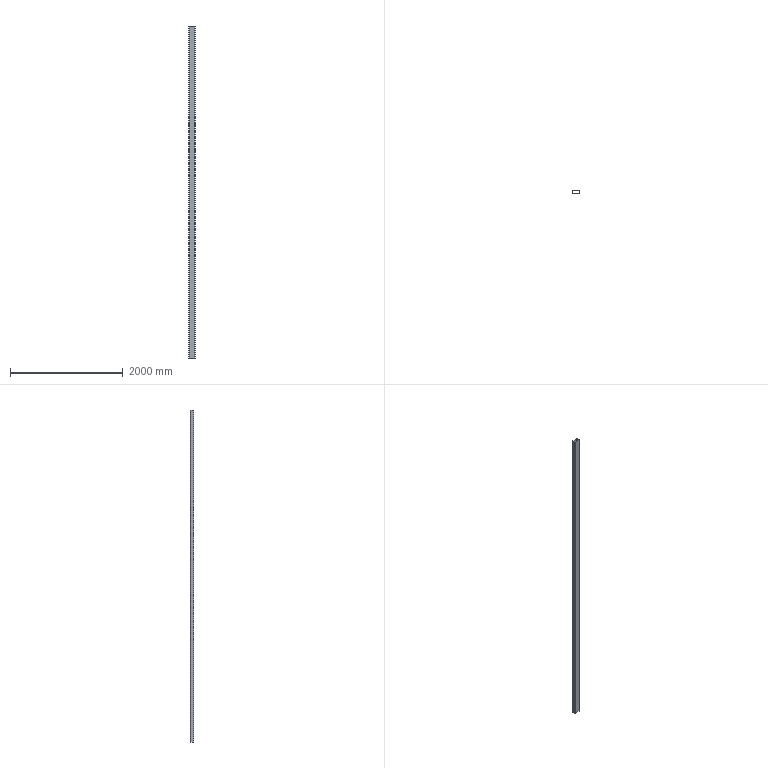Part | SolidWorks | features Extrusion 1 | 1 solid | 18 faces | box 120 x 60 x 5880 mm | volume 9617442 mm3 | plane 10 | cylinder 8 | commonest cylinder face diameters 10 x4 20 x4
STEP:
#1=CARTESIAN_POINT('',(110.,0.,5880.));
#2=VERTEX_POINT('',#1);
#3=CARTESIAN_POINT('',(120.,10.,5880.));
#4=VERTEX_POINT('',#3);
#5=CARTESIAN_POINT('',(110.,10.,5880.));
#6=DIRECTION('',(0.,0.,1.));
#7=DIRECTION('',(-1.,0.,0.));
#8=AXIS2_PLACEMENT_3D('',#5,#6,#7);
#9=CIRCLE('',#8,10.);
#10=EDGE_CURVE('',#2,#4,#9,.T.);
#11=ORIENTED_EDGE('',*,*,#10,.T.);
#12=CARTESIAN_POINT('',(120.,50.,5880.));
#13=VERTEX_POINT('',#12);
#14=CARTESIAN_POINT('',(120.,10.,5880.));
#15=DIRECTION('',(0.,1.,0.));
#16=VECTOR('',#15,1000.);
#17=LINE('',#14,#16);
#18=EDGE_CURVE('',#4,#13,#17,.T.);
#19=ORIENTED_EDGE('',*,*,#18,.T.);
#20=CARTESIAN_POINT('',(110.,60.,5880.));
#21=VERTEX_POINT('',#20);
#22=CARTESIAN_POINT('',(110.,50.,5880.));
#23=DIRECTION('',(0.,0.,1.));
#24=DIRECTION('',(1.,0.,0.));
#25=AXIS2_PLACEMENT_3D('',#22,#23,#24);
#26=CIRCLE('',#25,10.);
#27=EDGE_CURVE('',#13,#21,#26,.T.);
#28=ORIENTED_EDGE('',*,*,#27,.T.);
#29=CARTESIAN_POINT('',(10.,60.,5880.));
#30=VERTEX_POINT('',#29);
#31=CARTESIAN_POINT('',(10.,60.,5880.));
#32=DIRECTION('',(-1.,0.,0.));
#33=VECTOR('',#32,1000.);
#34=LINE('',#31,#33);
#35=EDGE_CURVE('',#21,#30,#34,.T.);
#36=ORIENTED_EDGE('',*,*,#35,.T.);
#37=CARTESIAN_POINT('',(0.,50.,5880.));
#38=VERTEX_POINT('',#37);
#39=CARTESIAN_POINT('',(10.,50.,5880.));
#40=DIRECTION('',(0.,0.,1.));
#41=DIRECTION('',(-1.,0.,0.));
#42=AXIS2_PLACEMENT_3D('',#39,#40,#41);
#43=CIRCLE('',#42,10.);
#44=EDGE_CURVE('',#30,#38,#43,.T.);
#45=ORIENTED_EDGE('',*,*,#44,.T.);
#46=CARTESIAN_POINT('',(0.,10.,5880.));
#47=VERTEX_POINT('',#46);
#48=CARTESIAN_POINT('',(0.,10.,5880.));
#49=DIRECTION('',(0.,-1.,0.));
#50=VECTOR('',#49,1000.);
#51=LINE('',#48,#50);
#52=EDGE_CURVE('',#38,#47,#51,.T.);
#53=ORIENTED_EDGE('',*,*,#52,.T.);
#54=CARTESIAN_POINT('',(10.,0.,5880.));
#55=VERTEX_POINT('',#54);
#56=CARTESIAN_POINT('',(10.,10.,5880.));
#57=DIRECTION('',(0.,0.,1.));
#58=DIRECTION('',(-1.,0.,0.));
#59=AXIS2_PLACEMENT_3D('',#56,#57,#58);
#60=CIRCLE('',#59,10.);
#61=EDGE_CURVE('',#47,#55,#60,.T.);
#62=ORIENTED_EDGE('',*,*,#61,.T.);
#63=CARTESIAN_POINT('',(10.,0.,5880.));
#64=DIRECTION('',(1.,0.,0.));
#65=VECTOR('',#64,1000.);
#66=LINE('',#63,#65);
#67=EDGE_CURVE('',#55,#2,#66,.T.);
#68=ORIENTED_EDGE('',*,*,#67,.T.);
#69=EDGE_LOOP('',(#11,#19,#28,#36,#45,#53,#62,#68));
#70=FACE_OUTER_BOUND('',#69,.T.);
#71=CARTESIAN_POINT('',(10.,55.,5880.));
#72=VERTEX_POINT('',#71);
#73=CARTESIAN_POINT('',(5.,50.,5880.));
#74=VERTEX_POINT('',#73);
#75=CARTESIAN_POINT('',(10.,50.,5880.));
#76=DIRECTION('',(0.,0.,1.));
#77=DIRECTION('',(-1.,0.,0.));
#78=AXIS2_PLACEMENT_3D('',#75,#76,#77);
#79=CIRCLE('',#78,5.);
#80=EDGE_CURVE('',#72,#74,#79,.T.);
#81=ORIENTED_EDGE('',*,*,#80,.F.);
#82=CARTESIAN_POINT('',(110.,55.,5880.));
#83=VERTEX_POINT('',#82);
#84=CARTESIAN_POINT('',(10.,55.,5880.));
#85=DIRECTION('',(-1.,0.,0.));
#86=VECTOR('',#85,1000.);
#87=LINE('',#84,#86);
#88=EDGE_CURVE('',#83,#72,#87,.T.);
#89=ORIENTED_EDGE('',*,*,#88,.F.);
#90=CARTESIAN_POINT('',(115.,50.,5880.));
#91=VERTEX_POINT('',#90);
#92=CARTESIAN_POINT('',(110.,50.,5880.));
#93=DIRECTION('',(0.,0.,1.));
#94=DIRECTION('',(1.,0.,0.));
#95=AXIS2_PLACEMENT_3D('',#92,#93,#94);
#96=CIRCLE('',#95,5.);
#97=EDGE_CURVE('',#91,#83,#96,.T.);
#98=ORIENTED_EDGE('',*,*,#97,.F.);
#99=CARTESIAN_POINT('',(115.,10.,5880.));
#100=VERTEX_POINT('',#99);
#101=CARTESIAN_POINT('',(115.,10.,5880.));
#102=DIRECTION('',(0.,1.,0.));
#103=VECTOR('',#102,1000.);
#104=LINE('',#101,#103);
#105=EDGE_CURVE('',#100,#91,#104,.T.);
#106=ORIENTED_EDGE('',*,*,#105,.F.);
#107=CARTESIAN_POINT('',(110.,5.,5880.));
#108=VERTEX_POINT('',#107);
#109=CARTESIAN_POINT('',(110.,10.,5880.));
#110=DIRECTION('',(0.,0.,1.));
#111=DIRECTION('',(-1.,0.,0.));
#112=AXIS2_PLACEMENT_3D('',#109,#110,#111);
#113=CIRCLE('',#112,5.);
#114=EDGE_CURVE('',#108,#100,#113,.T.);
#115=ORIENTED_EDGE('',*,*,#114,.F.);
#116=CARTESIAN_POINT('',(10.,5.,5880.));
#117=VERTEX_POINT('',#116);
#118=CARTESIAN_POINT('',(10.,5.,5880.));
#119=DIRECTION('',(1.,0.,0.));
#120=VECTOR('',#119,1000.);
#121=LINE('',#118,#120);
#122=EDGE_CURVE('',#117,#108,#121,.T.);
#123=ORIENTED_EDGE('',*,*,#122,.F.);
#124=CARTESIAN_POINT('',(5.,10.,5880.));
#125=VERTEX_POINT('',#124);
#126=CARTESIAN_POINT('',(10.,10.,5880.));
#127=DIRECTION('',(0.,0.,1.));
#128=DIRECTION('',(-1.,0.,0.));
#129=AXIS2_PLACEMENT_3D('',#126,#127,#128);
#130=CIRCLE('',#129,5.);
#131=EDGE_CURVE('',#125,#117,#130,.T.);
#132=ORIENTED_EDGE('',*,*,#131,.F.);
#133=CARTESIAN_POINT('',(5.,10.,5880.));
#134=DIRECTION('',(0.,-1.,0.));
#135=VECTOR('',#134,1000.);
#136=LINE('',#133,#135);
#137=EDGE_CURVE('',#74,#125,#136,.T.);
#138=ORIENTED_EDGE('',*,*,#137,.F.);
#139=EDGE_LOOP('',(#81,#89,#98,#106,#115,#123,#132,#138));
#140=FACE_BOUND('',#139,.T.);
#141=CARTESIAN_POINT('',(110.,10.,5880.));
#142=DIRECTION('',(0.,0.,-1.));
#143=DIRECTION('',(-1.,0.,0.));
#144=AXIS2_PLACEMENT_3D('',#141,#142,#143);
#145=PLANE('',#144);
#146=ADVANCED_FACE('',(#70,#140),#145,.F.);
#147=CARTESIAN_POINT('',(110.,0.,0.));
#148=VERTEX_POINT('',#147);
#149=CARTESIAN_POINT('',(120.,10.,0.));
#150=VERTEX_POINT('',#149);
#151=CARTESIAN_POINT('',(110.,10.,0.));
#152=DIRECTION('',(0.,0.,1.));
#153=DIRECTION('',(-1.,0.,0.));
#154=AXIS2_PLACEMENT_3D('',#151,#152,#153);
#155=CIRCLE('',#154,10.);
#156=EDGE_CURVE('',#148,#150,#155,.T.);
#157=ORIENTED_EDGE('',*,*,#156,.F.);
#158=CARTESIAN_POINT('',(10.,0.,0.));
#159=VERTEX_POINT('',#158);
#160=CARTESIAN_POINT('',(10.,0.,0.));
#161=DIRECTION('',(1.,0.,0.));
#162=VECTOR('',#161,1000.);
#163=LINE('',#160,#162);
#164=EDGE_CURVE('',#159,#148,#163,.T.);
#165=ORIENTED_EDGE('',*,*,#164,.F.);
#166=CARTESIAN_POINT('',(0.,10.,0.));
#167=VERTEX_POINT('',#166);
#168=CARTESIAN_POINT('',(10.,10.,0.));
#169=DIRECTION('',(0.,0.,1.));
#170=DIRECTION('',(-1.,0.,0.));
#171=AXIS2_PLACEMENT_3D('',#168,#169,#170);
#172=CIRCLE('',#171,10.);
#173=EDGE_CURVE('',#167,#159,#172,.T.);
#174=ORIENTED_EDGE('',*,*,#173,.F.);
#175=CARTESIAN_POINT('',(0.,50.,0.));
#176=VERTEX_POINT('',#175);
#177=CARTESIAN_POINT('',(0.,10.,0.));
#178=DIRECTION('',(0.,-1.,0.));
#179=VECTOR('',#178,1000.);
#180=LINE('',#177,#179);
#181=EDGE_CURVE('',#176,#167,#180,.T.);
#182=ORIENTED_EDGE('',*,*,#181,.F.);
#183=CARTESIAN_POINT('',(10.,60.,0.));
#184=VERTEX_POINT('',#183);
#185=CARTESIAN_POINT('',(10.,50.,0.));
#186=DIRECTION('',(0.,0.,1.));
#187=DIRECTION('',(-1.,0.,0.));
#188=AXIS2_PLACEMENT_3D('',#185,#186,#187);
#189=CIRCLE('',#188,10.);
#190=EDGE_CURVE('',#184,#176,#189,.T.);
#191=ORIENTED_EDGE('',*,*,#190,.F.);
#192=CARTESIAN_POINT('',(110.,60.,0.));
#193=VERTEX_POINT('',#192);
#194=CARTESIAN_POINT('',(10.,60.,0.));
#195=DIRECTION('',(-1.,0.,0.));
#196=VECTOR('',#195,1000.);
#197=LINE('',#194,#196);
#198=EDGE_CURVE('',#193,#184,#197,.T.);
#199=ORIENTED_EDGE('',*,*,#198,.F.);
#200=CARTESIAN_POINT('',(120.,50.,0.));
#201=VERTEX_POINT('',#200);
#202=CARTESIAN_POINT('',(110.,50.,0.));
#203=DIRECTION('',(0.,0.,1.));
#204=DIRECTION('',(1.,0.,0.));
#205=AXIS2_PLACEMENT_3D('',#202,#203,#204);
#206=CIRCLE('',#205,10.);
#207=EDGE_CURVE('',#201,#193,#206,.T.);
#208=ORIENTED_EDGE('',*,*,#207,.F.);
#209=CARTESIAN_POINT('',(120.,10.,0.));
#210=DIRECTION('',(0.,1.,0.));
#211=VECTOR('',#210,1000.);
#212=LINE('',#209,#211);
#213=EDGE_CURVE('',#150,#201,#212,.T.);
#214=ORIENTED_EDGE('',*,*,#213,.F.);
#215=EDGE_LOOP('',(#157,#165,#174,#182,#191,#199,#208,#214));
#216=FACE_OUTER_BOUND('',#215,.T.);
#217=CARTESIAN_POINT('',(110.,55.,0.));
#218=VERTEX_POINT('',#217);
#219=CARTESIAN_POINT('',(10.,55.,0.));
#220=VERTEX_POINT('',#219);
#221=CARTESIAN_POINT('',(10.,55.,0.));
#222=DIRECTION('',(-1.,0.,0.));
#223=VECTOR('',#222,1000.);
#224=LINE('',#221,#223);
#225=EDGE_CURVE('',#218,#220,#224,.T.);
#226=ORIENTED_EDGE('',*,*,#225,.T.);
#227=CARTESIAN_POINT('',(5.,50.,0.));
#228=VERTEX_POINT('',#227);
#229=CARTESIAN_POINT('',(10.,50.,0.));
#230=DIRECTION('',(0.,0.,1.));
#231=DIRECTION('',(-1.,0.,0.));
#232=AXIS2_PLACEMENT_3D('',#229,#230,#231);
#233=CIRCLE('',#232,5.);
#234=EDGE_CURVE('',#220,#228,#233,.T.);
#235=ORIENTED_EDGE('',*,*,#234,.T.);
#236=CARTESIAN_POINT('',(5.,10.,0.));
#237=VERTEX_POINT('',#236);
#238=CARTESIAN_POINT('',(5.,10.,0.));
#239=DIRECTION('',(0.,-1.,0.));
#240=VECTOR('',#239,1000.);
#241=LINE('',#238,#240);
#242=EDGE_CURVE('',#228,#237,#241,.T.);
#243=ORIENTED_EDGE('',*,*,#242,.T.);
#244=CARTESIAN_POINT('',(10.,5.,0.));
#245=VERTEX_POINT('',#244);
#246=CARTESIAN_POINT('',(10.,10.,0.));
#247=DIRECTION('',(0.,0.,1.));
#248=DIRECTION('',(-1.,0.,0.));
#249=AXIS2_PLACEMENT_3D('',#246,#247,#248);
#250=CIRCLE('',#249,5.);
#251=EDGE_CURVE('',#237,#245,#250,.T.);
#252=ORIENTED_EDGE('',*,*,#251,.T.);
#253=CARTESIAN_POINT('',(110.,5.,0.));
#254=VERTEX_POINT('',#253);
#255=CARTESIAN_POINT('',(10.,5.,0.));
#256=DIRECTION('',(1.,0.,0.));
#257=VECTOR('',#256,1000.);
#258=LINE('',#255,#257);
#259=EDGE_CURVE('',#245,#254,#258,.T.);
#260=ORIENTED_EDGE('',*,*,#259,.T.);
#261=CARTESIAN_POINT('',(115.,10.,0.));
#262=VERTEX_POINT('',#261);
#263=CARTESIAN_POINT('',(110.,10.,0.));
#264=DIRECTION('',(0.,0.,1.));
#265=DIRECTION('',(-1.,0.,0.));
#266=AXIS2_PLACEMENT_3D('',#263,#264,#265);
#267=CIRCLE('',#266,5.);
#268=EDGE_CURVE('',#254,#262,#267,.T.);
#269=ORIENTED_EDGE('',*,*,#268,.T.);
#270=CARTESIAN_POINT('',(115.,50.,0.));
#271=VERTEX_POINT('',#270);
#272=CARTESIAN_POINT('',(115.,10.,0.));
#273=DIRECTION('',(0.,1.,0.));
#274=VECTOR('',#273,1000.);
#275=LINE('',#272,#274);
#276=EDGE_CURVE('',#262,#271,#275,.T.);
#277=ORIENTED_EDGE('',*,*,#276,.T.);
#278=CARTESIAN_POINT('',(110.,50.,0.));
#279=DIRECTION('',(0.,0.,1.));
#280=DIRECTION('',(1.,0.,0.));
#281=AXIS2_PLACEMENT_3D('',#278,#279,#280);
#282=CIRCLE('',#281,5.);
#283=EDGE_CURVE('',#271,#218,#282,.T.);
#284=ORIENTED_EDGE('',*,*,#283,.T.);
#285=EDGE_LOOP('',(#226,#235,#243,#252,#260,#269,#277,#284));
#286=FACE_BOUND('',#285,.T.);
#287=CARTESIAN_POINT('',(110.,10.,0.));
#288=DIRECTION('',(0.,0.,-1.));
#289=DIRECTION('',(-1.,0.,0.));
#290=AXIS2_PLACEMENT_3D('',#287,#288,#289);
#291=PLANE('',#290);
#292=ADVANCED_FACE('',(#216,#286),#291,.T.);
#293=ORIENTED_EDGE('',*,*,#156,.T.);
#294=CARTESIAN_POINT('',(120.,10.,5880.));
#295=DIRECTION('',(0.,0.,-1.));
#296=VECTOR('',#295,1000.);
#297=LINE('',#294,#296);
#298=EDGE_CURVE('',#4,#150,#297,.T.);
#299=ORIENTED_EDGE('',*,*,#298,.F.);
#300=ORIENTED_EDGE('',*,*,#10,.F.);
#301=CARTESIAN_POINT('',(110.,0.,5880.));
#302=DIRECTION('',(0.,0.,-1.));
#303=VECTOR('',#302,1000.);
#304=LINE('',#301,#303);
#305=EDGE_CURVE('',#2,#148,#304,.T.);
#306=ORIENTED_EDGE('',*,*,#305,.T.);
#307=EDGE_LOOP('',(#293,#299,#300,#306));
#308=FACE_OUTER_BOUND('',#307,.T.);
#309=CARTESIAN_POINT('',(110.,10.,5880.));
#310=DIRECTION('',(0.,0.,-1.));
#311=DIRECTION('',(-1.,0.,0.));
#312=AXIS2_PLACEMENT_3D('',#309,#310,#311);
#313=CYLINDRICAL_SURFACE('',#312,10.);
#314=ADVANCED_FACE('',(#308),#313,.T.);
#315=ORIENTED_EDGE('',*,*,#213,.T.);
#316=CARTESIAN_POINT('',(120.,50.,5880.));
#317=DIRECTION('',(0.,0.,-1.));
#318=VECTOR('',#317,1000.);
#319=LINE('',#316,#318);
#320=EDGE_CURVE('',#13,#201,#319,.T.);
#321=ORIENTED_EDGE('',*,*,#320,.F.);
#322=ORIENTED_EDGE('',*,*,#18,.F.);
#323=ORIENTED_EDGE('',*,*,#298,.T.);
#324=EDGE_LOOP('',(#315,#321,#322,#323));
#325=FACE_OUTER_BOUND('',#324,.T.);
#326=CARTESIAN_POINT('',(120.,10.,5880.));
#327=DIRECTION('',(-1.,0.,0.));
#328=DIRECTION('',(0.,-1.,0.));
#329=AXIS2_PLACEMENT_3D('',#326,#327,#328);
#330=PLANE('',#329);
#331=ADVANCED_FACE('',(#325),#330,.F.);
#332=ORIENTED_EDGE('',*,*,#207,.T.);
#333=CARTESIAN_POINT('',(110.,60.,5880.));
#334=DIRECTION('',(0.,0.,-1.));
#335=VECTOR('',#334,1000.);
#336=LINE('',#333,#335);
#337=EDGE_CURVE('',#21,#193,#336,.T.);
#338=ORIENTED_EDGE('',*,*,#337,.F.);
#339=ORIENTED_EDGE('',*,*,#27,.F.);
#340=ORIENTED_EDGE('',*,*,#320,.T.);
#341=EDGE_LOOP('',(#332,#338,#339,#340));
#342=FACE_OUTER_BOUND('',#341,.T.);
#343=CARTESIAN_POINT('',(110.,50.,5880.));
#344=DIRECTION('',(0.,0.,-1.));
#345=DIRECTION('',(-1.,0.,0.));
#346=AXIS2_PLACEMENT_3D('',#343,#344,#345);
#347=CYLINDRICAL_SURFACE('',#346,10.);
#348=ADVANCED_FACE('',(#342),#347,.T.);
#349=ORIENTED_EDGE('',*,*,#198,.T.);
#350=CARTESIAN_POINT('',(10.,60.,5880.));
#351=DIRECTION('',(0.,0.,-1.));
#352=VECTOR('',#351,1000.);
#353=LINE('',#350,#352);
#354=EDGE_CURVE('',#30,#184,#353,.T.);
#355=ORIENTED_EDGE('',*,*,#354,.F.);
#356=ORIENTED_EDGE('',*,*,#35,.F.);
#357=ORIENTED_EDGE('',*,*,#337,.T.);
#358=EDGE_LOOP('',(#349,#355,#356,#357));
#359=FACE_OUTER_BOUND('',#358,.T.);
#360=CARTESIAN_POINT('',(10.,60.,5880.));
#361=DIRECTION('',(0.,-1.,0.));
#362=DIRECTION('',(0.,0.,-1.));
#363=AXIS2_PLACEMENT_3D('',#360,#361,#362);
#364=PLANE('',#363);
#365=ADVANCED_FACE('',(#359),#364,.F.);
#366=ORIENTED_EDGE('',*,*,#190,.T.);
#367=CARTESIAN_POINT('',(0.,50.,5880.));
#368=DIRECTION('',(0.,0.,-1.));
#369=VECTOR('',#368,1000.);
#370=LINE('',#367,#369);
#371=EDGE_CURVE('',#38,#176,#370,.T.);
#372=ORIENTED_EDGE('',*,*,#371,.F.);
#373=ORIENTED_EDGE('',*,*,#44,.F.);
#374=ORIENTED_EDGE('',*,*,#354,.T.);
#375=EDGE_LOOP('',(#366,#372,#373,#374));
#376=FACE_OUTER_BOUND('',#375,.T.);
#377=CARTESIAN_POINT('',(10.,50.,5880.));
#378=DIRECTION('',(0.,0.,-1.));
#379=DIRECTION('',(-1.,0.,0.));
#380=AXIS2_PLACEMENT_3D('',#377,#378,#379);
#381=CYLINDRICAL_SURFACE('',#380,10.);
#382=ADVANCED_FACE('',(#376),#381,.T.);
#383=ORIENTED_EDGE('',*,*,#181,.T.);
#384=CARTESIAN_POINT('',(0.,10.,5880.));
#385=DIRECTION('',(0.,0.,-1.));
#386=VECTOR('',#385,1000.);
#387=LINE('',#384,#386);
#388=EDGE_CURVE('',#47,#167,#387,.T.);
#389=ORIENTED_EDGE('',*,*,#388,.F.);
#390=ORIENTED_EDGE('',*,*,#52,.F.);
#391=ORIENTED_EDGE('',*,*,#371,.T.);
#392=EDGE_LOOP('',(#383,#389,#390,#391));
#393=FACE_OUTER_BOUND('',#392,.T.);
#394=CARTESIAN_POINT('',(0.,10.,5880.));
#395=DIRECTION('',(1.,0.,0.));
#396=DIRECTION('',(0.,1.,0.));
#397=AXIS2_PLACEMENT_3D('',#394,#395,#396);
#398=PLANE('',#397);
#399=ADVANCED_FACE('',(#393),#398,.F.);
#400=ORIENTED_EDGE('',*,*,#173,.T.);
#401=CARTESIAN_POINT('',(10.,0.,5880.));
#402=DIRECTION('',(0.,0.,-1.));
#403=VECTOR('',#402,1000.);
#404=LINE('',#401,#403);
#405=EDGE_CURVE('',#55,#159,#404,.T.);
#406=ORIENTED_EDGE('',*,*,#405,.F.);
#407=ORIENTED_EDGE('',*,*,#61,.F.);
#408=ORIENTED_EDGE('',*,*,#388,.T.);
#409=EDGE_LOOP('',(#400,#406,#407,#408));
#410=FACE_OUTER_BOUND('',#409,.T.);
#411=CARTESIAN_POINT('',(10.,10.,5880.));
#412=DIRECTION('',(0.,0.,-1.));
#413=DIRECTION('',(-1.,0.,0.));
#414=AXIS2_PLACEMENT_3D('',#411,#412,#413);
#415=CYLINDRICAL_SURFACE('',#414,10.);
#416=ADVANCED_FACE('',(#410),#415,.T.);
#417=ORIENTED_EDGE('',*,*,#164,.T.);
#418=ORIENTED_EDGE('',*,*,#305,.F.);
#419=ORIENTED_EDGE('',*,*,#67,.F.);
#420=ORIENTED_EDGE('',*,*,#405,.T.);
#421=EDGE_LOOP('',(#417,#418,#419,#420));
#422=FACE_OUTER_BOUND('',#421,.T.);
#423=CARTESIAN_POINT('',(10.,0.,5880.));
#424=DIRECTION('',(0.,1.,0.));
#425=DIRECTION('',(0.,0.,1.));
#426=AXIS2_PLACEMENT_3D('',#423,#424,#425);
#427=PLANE('',#426);
#428=ADVANCED_FACE('',(#422),#427,.F.);
#429=ORIENTED_EDGE('',*,*,#234,.F.);
#430=CARTESIAN_POINT('',(10.,55.,5880.));
#431=DIRECTION('',(0.,0.,-1.));
#432=VECTOR('',#431,1000.);
#433=LINE('',#430,#432);
#434=EDGE_CURVE('',#72,#220,#433,.T.);
#435=ORIENTED_EDGE('',*,*,#434,.F.);
#436=ORIENTED_EDGE('',*,*,#80,.T.);
#437=CARTESIAN_POINT('',(5.,50.,5880.));
#438=DIRECTION('',(0.,0.,-1.));
#439=VECTOR('',#438,1000.);
#440=LINE('',#437,#439);
#441=EDGE_CURVE('',#74,#228,#440,.T.);
#442=ORIENTED_EDGE('',*,*,#441,.T.);
#443=EDGE_LOOP('',(#429,#435,#436,#442));
#444=FACE_OUTER_BOUND('',#443,.T.);
#445=CARTESIAN_POINT('',(10.,50.,5880.));
#446=DIRECTION('',(0.,0.,-1.));
#447=DIRECTION('',(-1.,0.,0.));
#448=AXIS2_PLACEMENT_3D('',#445,#446,#447);
#449=CYLINDRICAL_SURFACE('',#448,5.);
#450=ADVANCED_FACE('',(#444),#449,.F.);
#451=ORIENTED_EDGE('',*,*,#242,.F.);
#452=ORIENTED_EDGE('',*,*,#441,.F.);
#453=ORIENTED_EDGE('',*,*,#137,.T.);
#454=CARTESIAN_POINT('',(5.,10.,5880.));
#455=DIRECTION('',(0.,0.,-1.));
#456=VECTOR('',#455,1000.);
#457=LINE('',#454,#456);
#458=EDGE_CURVE('',#125,#237,#457,.T.);
#459=ORIENTED_EDGE('',*,*,#458,.T.);
#460=EDGE_LOOP('',(#451,#452,#453,#459));
#461=FACE_OUTER_BOUND('',#460,.T.);
#462=CARTESIAN_POINT('',(5.,10.,5880.));
#463=DIRECTION('',(1.,0.,0.));
#464=DIRECTION('',(0.,1.,0.));
#465=AXIS2_PLACEMENT_3D('',#462,#463,#464);
#466=PLANE('',#465);
#467=ADVANCED_FACE('',(#461),#466,.T.);
#468=ORIENTED_EDGE('',*,*,#251,.F.);
#469=ORIENTED_EDGE('',*,*,#458,.F.);
#470=ORIENTED_EDGE('',*,*,#131,.T.);
#471=CARTESIAN_POINT('',(10.,5.,5880.));
#472=DIRECTION('',(0.,0.,-1.));
#473=VECTOR('',#472,1000.);
#474=LINE('',#471,#473);
#475=EDGE_CURVE('',#117,#245,#474,.T.);
#476=ORIENTED_EDGE('',*,*,#475,.T.);
#477=EDGE_LOOP('',(#468,#469,#470,#476));
#478=FACE_OUTER_BOUND('',#477,.T.);
#479=CARTESIAN_POINT('',(10.,10.,5880.));
#480=DIRECTION('',(0.,0.,-1.));
#481=DIRECTION('',(-1.,0.,0.));
#482=AXIS2_PLACEMENT_3D('',#479,#480,#481);
#483=CYLINDRICAL_SURFACE('',#482,5.);
#484=ADVANCED_FACE('',(#478),#483,.F.);
#485=ORIENTED_EDGE('',*,*,#259,.F.);
#486=ORIENTED_EDGE('',*,*,#475,.F.);
#487=ORIENTED_EDGE('',*,*,#122,.T.);
#488=CARTESIAN_POINT('',(110.,5.,5880.));
#489=DIRECTION('',(0.,0.,-1.));
#490=VECTOR('',#489,1000.);
#491=LINE('',#488,#490);
#492=EDGE_CURVE('',#108,#254,#491,.T.);
#493=ORIENTED_EDGE('',*,*,#492,.T.);
#494=EDGE_LOOP('',(#485,#486,#487,#493));
#495=FACE_OUTER_BOUND('',#494,.T.);
#496=CARTESIAN_POINT('',(10.,5.,5880.));
#497=DIRECTION('',(0.,1.,0.));
#498=DIRECTION('',(0.,0.,1.));
#499=AXIS2_PLACEMENT_3D('',#496,#497,#498);
#500=PLANE('',#499);
#501=ADVANCED_FACE('',(#495),#500,.T.);
#502=ORIENTED_EDGE('',*,*,#268,.F.);
#503=ORIENTED_EDGE('',*,*,#492,.F.);
#504=ORIENTED_EDGE('',*,*,#114,.T.);
#505=CARTESIAN_POINT('',(115.,10.,5880.));
#506=DIRECTION('',(0.,0.,-1.));
#507=VECTOR('',#506,1000.);
#508=LINE('',#505,#507);
#509=EDGE_CURVE('',#100,#262,#508,.T.);
#510=ORIENTED_EDGE('',*,*,#509,.T.);
#511=EDGE_LOOP('',(#502,#503,#504,#510));
#512=FACE_OUTER_BOUND('',#511,.T.);
#513=CARTESIAN_POINT('',(110.,10.,5880.));
#514=DIRECTION('',(0.,0.,-1.));
#515=DIRECTION('',(-1.,0.,0.));
#516=AXIS2_PLACEMENT_3D('',#513,#514,#515);
#517=CYLINDRICAL_SURFACE('',#516,5.);
#518=ADVANCED_FACE('',(#512),#517,.F.);
#519=ORIENTED_EDGE('',*,*,#276,.F.);
#520=ORIENTED_EDGE('',*,*,#509,.F.);
#521=ORIENTED_EDGE('',*,*,#105,.T.);
#522=CARTESIAN_POINT('',(115.,50.,5880.));
#523=DIRECTION('',(0.,0.,-1.));
#524=VECTOR('',#523,1000.);
#525=LINE('',#522,#524);
#526=EDGE_CURVE('',#91,#271,#525,.T.);
#527=ORIENTED_EDGE('',*,*,#526,.T.);
#528=EDGE_LOOP('',(#519,#520,#521,#527));
#529=FACE_OUTER_BOUND('',#528,.T.);
#530=CARTESIAN_POINT('',(115.,10.,5880.));
#531=DIRECTION('',(-1.,0.,0.));
#532=DIRECTION('',(0.,0.,1.));
#533=AXIS2_PLACEMENT_3D('',#530,#531,#532);
#534=PLANE('',#533);
#535=ADVANCED_FACE('',(#529),#534,.T.);
#536=ORIENTED_EDGE('',*,*,#283,.F.);
#537=ORIENTED_EDGE('',*,*,#526,.F.);
#538=ORIENTED_EDGE('',*,*,#97,.T.);
#539=CARTESIAN_POINT('',(110.,55.,5880.));
#540=DIRECTION('',(0.,0.,-1.));
#541=VECTOR('',#540,1000.);
#542=LINE('',#539,#541);
#543=EDGE_CURVE('',#83,#218,#542,.T.);
#544=ORIENTED_EDGE('',*,*,#543,.T.);
#545=EDGE_LOOP('',(#536,#537,#538,#544));
#546=FACE_OUTER_BOUND('',#545,.T.);
#547=CARTESIAN_POINT('',(110.,50.,5880.));
#548=DIRECTION('',(0.,0.,-1.));
#549=DIRECTION('',(-1.,0.,0.));
#550=AXIS2_PLACEMENT_3D('',#547,#548,#549);
#551=CYLINDRICAL_SURFACE('',#550,5.);
#552=ADVANCED_FACE('',(#546),#551,.F.);
#553=ORIENTED_EDGE('',*,*,#225,.F.);
#554=ORIENTED_EDGE('',*,*,#543,.F.);
#555=ORIENTED_EDGE('',*,*,#88,.T.);
#556=ORIENTED_EDGE('',*,*,#434,.T.);
#557=EDGE_LOOP('',(#553,#554,#555,#556));
#558=FACE_OUTER_BOUND('',#557,.T.);
#559=CARTESIAN_POINT('',(10.,55.,5880.));
#560=DIRECTION('',(0.,-1.,0.));
#561=DIRECTION('',(0.,0.,-1.));
#562=AXIS2_PLACEMENT_3D('',#559,#560,#561);
#563=PLANE('',#562);
#564=ADVANCED_FACE('',(#558),#563,.T.);
#565=CLOSED_SHELL('',(#146,#292,#314,#331,#348,#365,#382,#399,#416,#428,#450,#467,#484,#501,#518,#535,#552,#564));
#566=MANIFOLD_SOLID_BREP('',#565);
#567=CARTESIAN_POINT('',(0.,0.,0.));
#568=DIRECTION('',(0.,0.,1.));
#569=DIRECTION('',(1.,0.,0.));
#570=AXIS2_PLACEMENT_3D('',#567,#568,#569);
#571=(LENGTH_UNIT()NAMED_UNIT(*)SI_UNIT(.MILLI.,.METRE.));
#572=UNCERTAINTY_MEASURE_WITH_UNIT(LENGTH_MEASURE(0.00001),#571,'','');
#573=(NAMED_UNIT(*)PLANE_ANGLE_UNIT()SI_UNIT($,.RADIAN.));
#574=(NAMED_UNIT(*)SI_UNIT($,.STERADIAN.)SOLID_ANGLE_UNIT());
#575=(GEOMETRIC_REPRESENTATION_CONTEXT(3)GLOBAL_UNCERTAINTY_ASSIGNED_CONTEXT((#572))GLOBAL_UNIT_ASSIGNED_CONTEXT((#571,#573,#574))REPRESENTATION_CONTEXT('',''));
#576=ADVANCED_BREP_SHAPE_REPRESENTATION('',(#566,#570),#575);